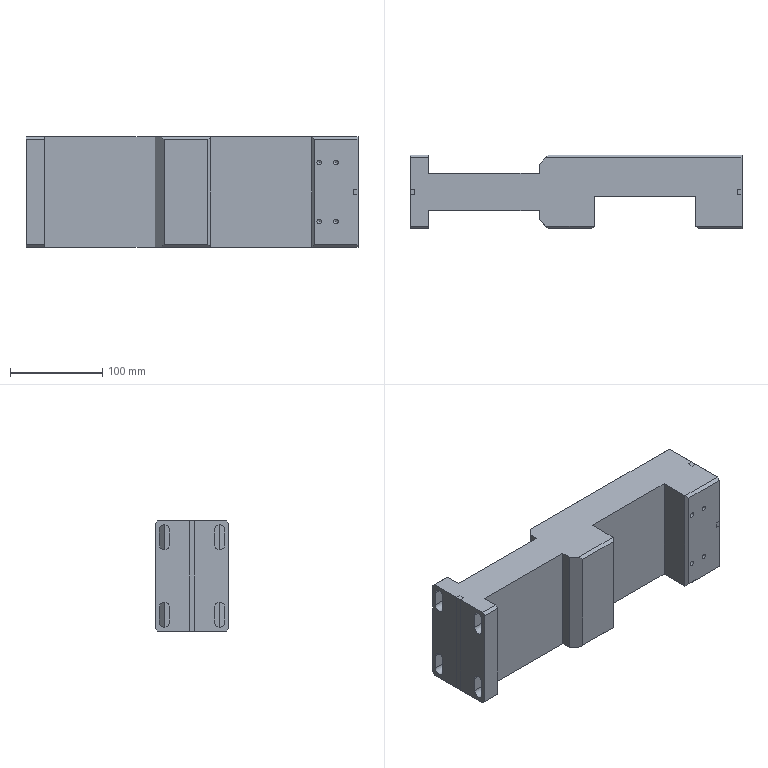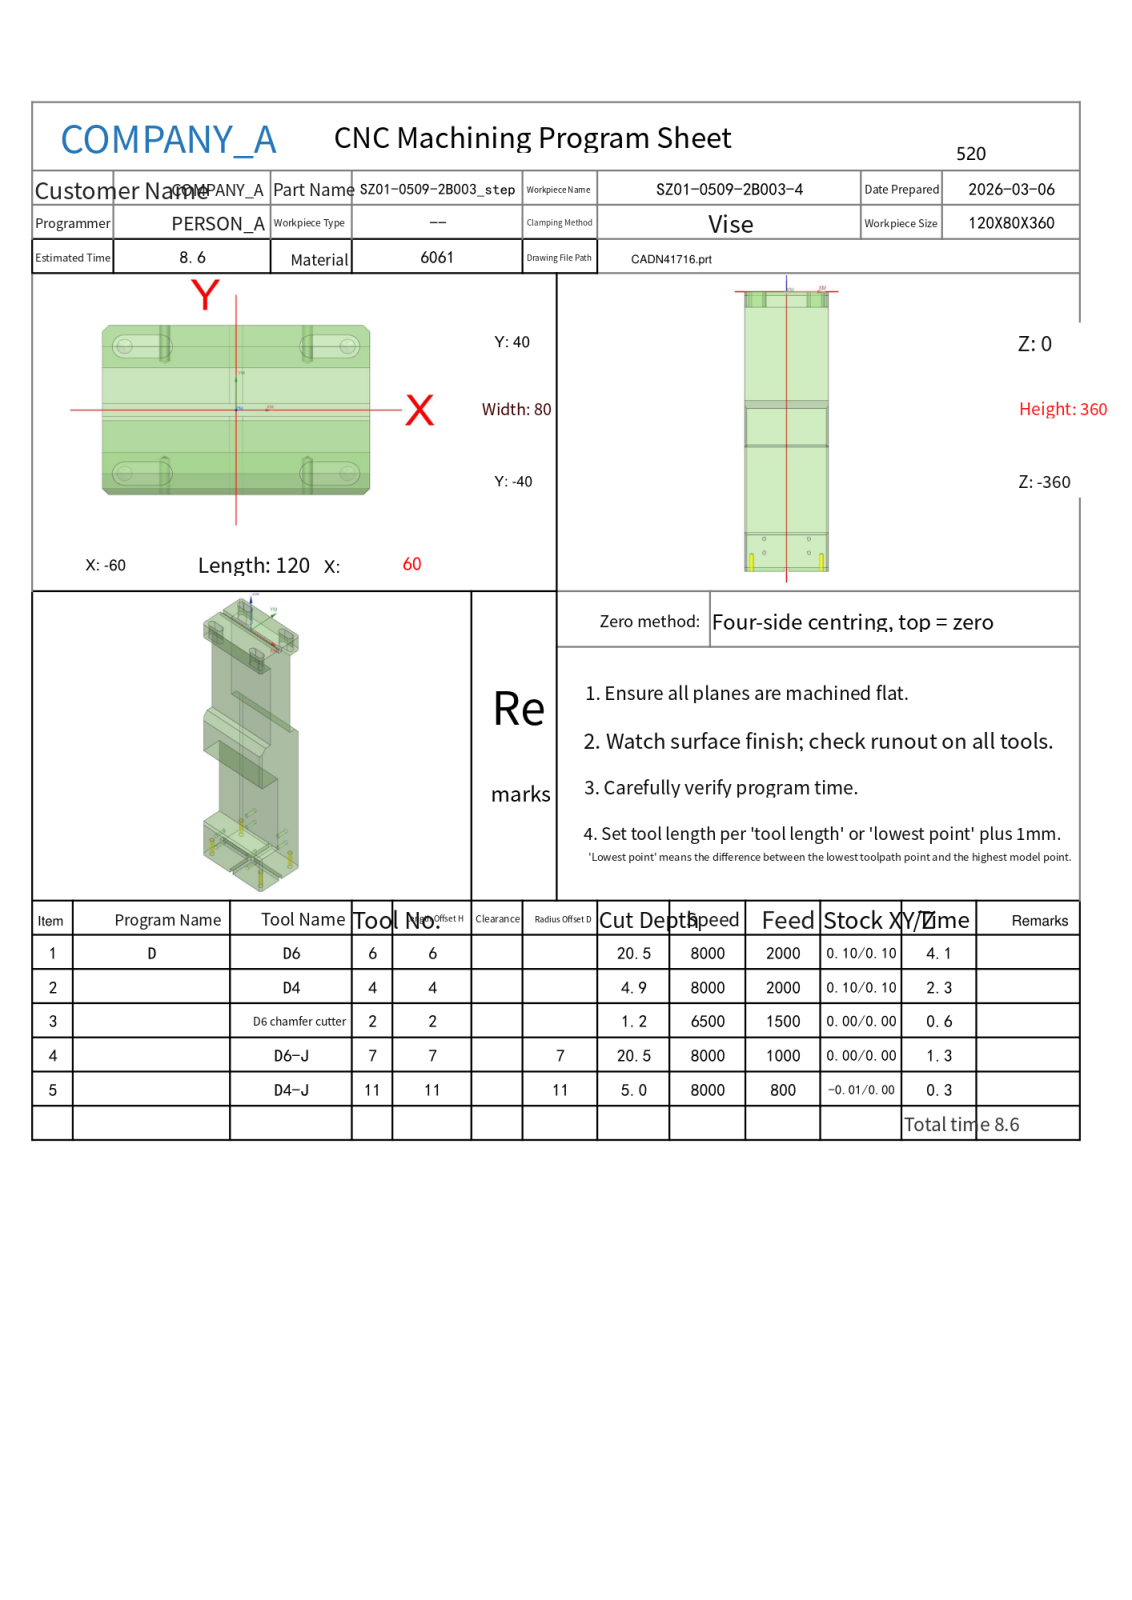NC program | NX | posted by the shop | part box 360 x 80 x 120 mm
Whole program, first 1404 of 1841 lines:
%
O0001
(Machine time: 9.60 MIN)
(===Total Tool:5===)
(T6=D6      D=6.   R=0.   D-  H06 Z=-20.5 )
(T4=D4      D=4.   R=0.   D-  H04 Z=-4.9  )
(T2=D6 chamfer cutter   D=6.   R=0.   D-  H02 Z=-1.2  )
(T7=D6-J    D=6.   R=0.   D7  H07 Z=-20.5 )
(T11=D4-J   D=4.   R=0.   D11 H11 Z=-5.   )
G80 G90 G17 G49 G40
G91 G28 Z0
M01
N1 T06 M06
(D6  D=6. R=0. H=06 ce=0.10 di=0.10)
G00 G90 G54 X-38.502 Y-27.6 M03 S8000
G43 H06 Z50.
M08
Z1.
G01 X-50.381 Z.377 F2000.
X-51.324 Y-27.962 Z.325
X-52.038 Y-28.676 Z.272
X-52.4 Y-29.619 Z.219
Y-30.381 Z.179
X-52.038 Y-31.324 Z.126
X-51.324 Y-32.038 Z.073
X-50.381 Y-32.4 Z.02
X-50. Z0.0
X-34. Z-.166
G03 X-31.6 Y-30. Z-.205 I0.0 J2.4
X-34. Y-27.6 Z-.244 I-2.4 J0.0
G01 X-50. Z-.41
G03 X-52.4 Y-30. Z-.449 I0.0 J-2.4
X-50. Y-32.4 Z-.488 I2.4 J0.0
G01 X-34. Z-.654
G03 X-31.6 Y-30. Z-.693 I0.0 J2.4
X-34. Y-27.6 Z-.732 I-2.4 J0.0
G01 X-50. Z-.898
G03 X-52.4 Y-30. Z-.937 I0.0 J-2.4
X-50. Y-32.4 Z-.976 I2.4 J0.0
G01 X-34. Z-1.142
G03 X-31.6 Y-30. Z-1.181 I0.0 J2.4
X-34. Y-27.6 Z-1.22 I-2.4 J0.0
G01 X-50. Z-1.386
G03 X-52.4 Y-30. Z-1.425 I0.0 J-2.4
X-50. Y-32.4 Z-1.464 I2.4 J0.0
G01 X-34. Z-1.63
G03 X-31.6 Y-30. Z-1.669 I0.0 J2.4
X-34. Y-27.6 Z-1.708 I-2.4 J0.0
G01 X-50. Z-1.874
G03 X-52.4 Y-30. Z-1.913 I0.0 J-2.4
X-50. Y-32.4 Z-1.952 I2.4 J0.0
G01 X-34. Z-2.118
G03 X-31.6 Y-30. Z-2.157 I0.0 J2.4
X-34. Y-27.6 Z-2.196 I-2.4 J0.0
G01 X-50. Z-2.362
G03 X-52.4 Y-30. Z-2.401 I0.0 J-2.4
X-50. Y-32.4 Z-2.44 I2.4 J0.0
G01 X-34. Z-2.606
G03 X-31.6 Y-30. Z-2.645 I0.0 J2.4
X-34. Y-27.6 Z-2.685 I-2.4 J0.0
G01 X-50. Z-2.85
G03 X-52.4 Y-30. Z-2.889 I0.0 J-2.4
X-50. Y-32.4 Z-2.929 I2.4 J0.0
G01 X-34. Z-3.094
G03 X-31.6 Y-30. Z-3.134 I0.0 J2.4
X-34. Y-27.6 Z-3.173 I-2.4 J0.0
G01 X-50. Z-3.338
G03 X-52.4 Y-30. Z-3.378 I0.0 J-2.4
X-50. Y-32.4 Z-3.417 I2.4 J0.0
G01 X-34. Z-3.583
G03 X-31.6 Y-30. Z-3.622 I0.0 J2.4
X-34. Y-27.6 Z-3.661 I-2.4 J0.0
G01 X-50. Z-3.827
G03 X-52.4 Y-30. Z-3.866 I0.0 J-2.4
X-50. Y-32.4 Z-3.905 I2.4 J0.0
G01 X-34. Z-4.071
G03 X-31.6 Y-30. Z-4.11 I0.0 J2.4
X-34. Y-27.6 Z-4.149 I-2.4 J0.0
G01 X-50. Z-4.315
G03 X-52.4 Y-30. Z-4.354 I0.0 J-2.4
X-50. Y-32.4 Z-4.393 I2.4 J0.0
G01 X-34. Z-4.559
G03 X-31.6 Y-30. Z-4.598 I0.0 J2.4
X-34. Y-27.6 Z-4.637 I-2.4 J0.0
G01 X-50. Z-4.803
G03 X-52.4 Y-30. Z-4.842 I0.0 J-2.4
X-50. Y-32.4 Z-4.881 I2.4 J0.0
G01 X-34. Z-5.047
G03 X-31.6 Y-30. Z-5.086 I0.0 J2.4
X-34. Y-27.6 Z-5.125 I-2.4 J0.0
G01 X-50. Z-5.291
G03 X-52.4 Y-30. Z-5.33 I0.0 J-2.4
X-50. Y-32.4 Z-5.369 I2.4 J0.0
G01 X-34. Z-5.535
G03 X-31.6 Y-30. Z-5.574 I0.0 J2.4
X-34. Y-27.6 Z-5.613 I-2.4 J0.0
G01 X-50. Z-5.779
G03 X-52.4 Y-30. Z-5.818 I0.0 J-2.4
X-50. Y-32.4 Z-5.857 I2.4 J0.0
G01 X-34. Z-6.023
G03 X-31.6 Y-30. Z-6.062 I0.0 J2.4
X-34. Y-27.6 Z-6.101 I-2.4 J0.0
G01 X-50. Z-6.267
G03 X-52.4 Y-30. Z-6.306 I0.0 J-2.4
X-50. Y-32.4 Z-6.345 I2.4 J0.0
G01 X-34. Z-6.511
G03 X-31.6 Y-30. Z-6.55 I0.0 J2.4
X-34. Y-27.6 Z-6.589 I-2.4 J0.0
G01 X-50. Z-6.755
G03 X-52.4 Y-30. Z-6.794 I0.0 J-2.4
X-50. Y-32.4 Z-6.833 I2.4 J0.0
G01 X-34. Z-6.999
G03 X-31.6 Y-30. Z-7.038 I0.0 J2.4
X-34. Y-27.6 Z-7.077 I-2.4 J0.0
G01 X-50. Z-7.243
G03 X-52.4 Y-30. Z-7.282 I0.0 J-2.4
X-50. Y-32.4 Z-7.321 I2.4 J0.0
G01 X-34. Z-7.487
G03 X-31.6 Y-30. Z-7.526 I0.0 J2.4
X-34. Y-27.6 Z-7.565 I-2.4 J0.0
G01 X-50. Z-7.731
G03 X-52.4 Y-30. Z-7.77 I0.0 J-2.4
X-50. Y-32.4 Z-7.81 I2.4 J0.0
G01 X-34. Z-7.975
G03 X-31.6 Y-30. Z-8.014 I0.0 J2.4
X-34. Y-27.6 Z-8.054 I-2.4 J0.0
G01 X-50. Z-8.219
G03 X-52.4 Y-30. Z-8.259 I0.0 J-2.4
X-50. Y-32.4 Z-8.298 I2.4 J0.0
G01 X-34. Z-8.463
G03 X-31.6 Y-30. Z-8.503 I0.0 J2.4
X-34. Y-27.6 Z-8.542 I-2.4 J0.0
G01 X-50. Z-8.708
G03 X-52.4 Y-30. Z-8.747 I0.0 J-2.4
X-50. Y-32.4 Z-8.786 I2.4 J0.0
G01 X-34. Z-8.952
G03 X-31.6 Y-30. Z-8.991 I0.0 J2.4
X-34. Y-27.6 Z-9.03 I-2.4 J0.0
G01 X-50. Z-9.196
G03 X-52.4 Y-30. Z-9.235 I0.0 J-2.4
X-50. Y-32.4 Z-9.274 I2.4 J0.0
G01 X-34. Z-9.44
G03 X-31.6 Y-30. Z-9.479 I0.0 J2.4
X-34. Y-27.6 Z-9.518 I-2.4 J0.0
G01 X-50. Z-9.684
G03 X-52.4 Y-30. Z-9.723 I0.0 J-2.4
X-50. Y-32.4 Z-9.762 I2.4 J0.0
G01 X-34. Z-9.928
G03 X-31.6 Y-30. Z-9.967 I0.0 J2.4
X-34. Y-27.6 Z-10.006 I-2.4 J0.0
G01 X-50. Z-10.172
G03 X-52.4 Y-30. Z-10.211 I0.0 J-2.4
X-50. Y-32.4 Z-10.25 I2.4 J0.0
G01 X-34. Z-10.416
G03 X-31.6 Y-30. Z-10.455 I0.0 J2.4
X-34. Y-27.6 Z-10.494 I-2.4 J0.0
G01 X-50. Z-10.66
G03 X-52.4 Y-30. Z-10.699 I0.0 J-2.4
X-50. Y-32.4 Z-10.738 I2.4 J0.0
G01 X-34. Z-10.904
G03 X-31.6 Y-30. Z-10.943 I0.0 J2.4
X-34. Y-27.6 Z-10.982 I-2.4 J0.0
G01 X-50. Z-11.148
G03 X-52.4 Y-30. Z-11.187 I0.0 J-2.4
X-50. Y-32.4 Z-11.226 I2.4 J0.0
G01 X-34. Z-11.392
G03 X-31.6 Y-30. Z-11.431 I0.0 J2.4
X-34. Y-27.6 Z-11.47 I-2.4 J0.0
G01 X-50. Z-11.636
G03 X-52.4 Y-30. Z-11.675 I0.0 J-2.4
X-50. Y-32.4 Z-11.714 I2.4 J0.0
G01 X-34. Z-11.88
G03 X-31.6 Y-30. Z-11.919 I0.0 J2.4
X-34. Y-27.6 Z-11.958 I-2.4 J0.0
G01 X-50. Z-12.124
G03 X-52.4 Y-30. Z-12.163 I0.0 J-2.4
X-50. Y-32.4 Z-12.202 I2.4 J0.0
G01 X-34. Z-12.368
G03 X-31.6 Y-30. Z-12.407 I0.0 J2.4
X-34. Y-27.6 Z-12.446 I-2.4 J0.0
G01 X-50. Z-12.612
G03 X-52.4 Y-30. Z-12.651 I0.0 J-2.4
X-50. Y-32.4 Z-12.69 I2.4 J0.0
G01 X-34. Z-12.856
G03 X-31.6 Y-30. Z-12.895 I0.0 J2.4
X-34. Y-27.6 Z-12.935 I-2.4 J0.0
G01 X-50. Z-13.1
G03 X-52.4 Y-30. Z-13.139 I0.0 J-2.4
X-50. Y-32.4 Z-13.179 I2.4 J0.0
G01 X-34. Z-13.344
G03 X-31.6 Y-30. Z-13.384 I0.0 J2.4
X-34. Y-27.6 Z-13.423 I-2.4 J0.0
G01 X-50. Z-13.588
G03 X-52.4 Y-30. Z-13.628 I0.0 J-2.4
X-50. Y-32.4 Z-13.667 I2.4 J0.0
G01 X-34. Z-13.833
G03 X-31.6 Y-30. Z-13.872 I0.0 J2.4
X-34. Y-27.6 Z-13.911 I-2.4 J0.0
G01 X-50. Z-14.077
G03 X-52.4 Y-30. Z-14.116 I0.0 J-2.4
X-50. Y-32.4 Z-14.155 I2.4 J0.0
G01 X-34. Z-14.321
G03 X-31.6 Y-30. Z-14.36 I0.0 J2.4
X-34. Y-27.6 Z-14.399 I-2.4 J0.0
G01 X-50. Z-14.565
G03 X-52.4 Y-30. Z-14.604 I0.0 J-2.4
X-50. Y-32.4 Z-14.643 I2.4 J0.0
G01 X-34. Z-14.809
G03 X-31.6 Y-30. Z-14.848 I0.0 J2.4
X-34. Y-27.6 Z-14.887 I-2.4 J0.0
G01 X-50. Z-15.053
G03 X-52.4 Y-30. Z-15.092 I0.0 J-2.4
X-50. Y-32.4 Z-15.131 I2.4 J0.0
G01 X-34. Z-15.297
G03 X-31.6 Y-30. Z-15.336 I0.0 J2.4
X-34. Y-27.6 Z-15.375 I-2.4 J0.0
G01 X-50. Z-15.541
G03 X-52.4 Y-30. Z-15.58 I0.0 J-2.4
X-50. Y-32.4 Z-15.619 I2.4 J0.0
G01 X-34. Z-15.785
G03 X-31.6 Y-30. Z-15.824 I0.0 J2.4
X-34. Y-27.6 Z-15.863 I-2.4 J0.0
G01 X-50. Z-16.029
G03 X-52.4 Y-30. Z-16.068 I0.0 J-2.4
X-50. Y-32.4 Z-16.107 I2.4 J0.0
G01 X-34. Z-16.273
G03 X-31.6 Y-30. Z-16.312 I0.0 J2.4
X-34. Y-27.6 Z-16.351 I-2.4 J0.0
G01 X-50. Z-16.517
G03 X-52.4 Y-30. Z-16.556 I0.0 J-2.4
X-50. Y-32.4 Z-16.595 I2.4 J0.0
G01 X-34. Z-16.761
G03 X-31.6 Y-30. Z-16.8 I0.0 J2.4
X-34. Y-27.6 Z-16.839 I-2.4 J0.0
G01 X-50. Z-17.005
G03 X-52.4 Y-30. Z-17.044 I0.0 J-2.4
X-50. Y-32.4 Z-17.083 I2.4 J0.0
G01 X-34. Z-17.249
G03 X-31.6 Y-30. Z-17.288 I0.0 J2.4
X-34. Y-27.6 Z-17.327 I-2.4 J0.0
G01 X-50. Z-17.493
G03 X-52.4 Y-30. Z-17.532 I0.0 J-2.4
X-50. Y-32.4 Z-17.571 I2.4 J0.0
G01 X-34. Z-17.737
G03 X-31.6 Y-30. Z-17.776 I0.0 J2.4
X-34. Y-27.6 Z-17.815 I-2.4 J0.0
G01 X-50. Z-17.981
G03 X-52.4 Y-30. Z-18.02 I0.0 J-2.4
X-50. Y-32.4 Z-18.06 I2.4 J0.0
G01 X-34. Z-18.225
G03 X-31.6 Y-30. Z-18.264 I0.0 J2.4
X-34. Y-27.6 Z-18.304 I-2.4 J0.0
G01 X-50. Z-18.469
G03 X-52.4 Y-30. Z-18.509 I0.0 J-2.4
X-50. Y-32.4 Z-18.548 I2.4 J0.0
G01 X-34. Z-18.713
G03 X-31.6 Y-30. Z-18.753 I0.0 J2.4
X-34. Y-27.6 Z-18.792 I-2.4 J0.0
G01 X-50. Z-18.958
G03 X-52.4 Y-30. Z-18.997 I0.0 J-2.4
X-50. Y-32.4 Z-19.036 I2.4 J0.0
G01 X-34. Z-19.202
G03 X-31.6 Y-30. Z-19.241 I0.0 J2.4
X-34. Y-27.6 Z-19.28 I-2.4 J0.0
G01 X-50. Z-19.446
G03 X-52.4 Y-30. Z-19.485 I0.0 J-2.4
X-50. Y-32.4 Z-19.524 I2.4 J0.0
G01 X-34. Z-19.69
G03 X-31.6 Y-30. Z-19.729 I0.0 J2.4
X-34. Y-27.6 Z-19.768 I-2.4 J0.0
G01 X-50. Z-19.934
G03 X-52.4 Y-30. Z-19.973 I0.0 J-2.4
X-50. Y-32.4 Z-20.012 I2.4 J0.0
G01 X-34. Z-20.178
G03 X-31.6 Y-30. Z-20.217 I0.0 J2.4
X-34. Y-27.6 Z-20.256 I-2.4 J0.0
G01 X-50. Z-20.422
G03 X-52.4 Y-30. Z-20.461 I0.0 J-2.4
X-50. Y-32.4 Z-20.5 I2.4 J0.0
G01 X-34.
G03 X-31.6 Y-30. I0.0 J2.4
X-34. Y-27.6 I-2.4 J0.0
G01 X-50.
G03 X-52.4 Y-30. I0.0 J-2.4
X-50. Y-32.4 I2.4 J0.0
G01 X-49.6
Z-19.5
G00 Z50.
X-45.498 Y27.6
Z1.
G01 X-33.619 Z.377
X-32.676 Y27.962 Z.325
X-31.962 Y28.676 Z.272
X-31.6 Y29.619 Z.219
Y30.381 Z.179
X-31.962 Y31.324 Z.126
X-32.676 Y32.038 Z.073
X-33.619 Y32.4 Z.02
X-34. Z0.0
X-50. Z-.166
G03 X-52.4 Y30. Z-.205 I0.0 J-2.4
X-50. Y27.6 Z-.244 I2.4 J0.0
G01 X-34. Z-.41
G03 X-31.6 Y30. Z-.449 I0.0 J2.4
X-34. Y32.4 Z-.488 I-2.4 J0.0
G01 X-50. Z-.654
G03 X-52.4 Y30. Z-.693 I0.0 J-2.4
X-50. Y27.6 Z-.732 I2.4 J0.0
G01 X-34. Z-.898
G03 X-31.6 Y30. Z-.937 I0.0 J2.4
X-34. Y32.4 Z-.976 I-2.4 J0.0
G01 X-50. Z-1.142
G03 X-52.4 Y30. Z-1.181 I0.0 J-2.4
X-50. Y27.6 Z-1.22 I2.4 J0.0
G01 X-34. Z-1.386
G03 X-31.6 Y30. Z-1.425 I0.0 J2.4
X-34. Y32.4 Z-1.464 I-2.4 J0.0
G01 X-50. Z-1.63
G03 X-52.4 Y30. Z-1.669 I0.0 J-2.4
X-50. Y27.6 Z-1.708 I2.4 J0.0
G01 X-34. Z-1.874
G03 X-31.6 Y30. Z-1.913 I0.0 J2.4
X-34. Y32.4 Z-1.952 I-2.4 J0.0
G01 X-50. Z-2.118
G03 X-52.4 Y30. Z-2.157 I0.0 J-2.4
X-50. Y27.6 Z-2.196 I2.4 J0.0
G01 X-34. Z-2.362
G03 X-31.6 Y30. Z-2.401 I0.0 J2.4
X-34. Y32.4 Z-2.44 I-2.4 J0.0
G01 X-50. Z-2.606
G03 X-52.4 Y30. Z-2.645 I0.0 J-2.4
X-50. Y27.6 Z-2.685 I2.4 J0.0
G01 X-34. Z-2.85
G03 X-31.6 Y30. Z-2.889 I0.0 J2.4
X-34. Y32.4 Z-2.929 I-2.4 J0.0
G01 X-50. Z-3.094
G03 X-52.4 Y30. Z-3.134 I0.0 J-2.4
X-50. Y27.6 Z-3.173 I2.4 J0.0
G01 X-34. Z-3.338
G03 X-31.6 Y30. Z-3.378 I0.0 J2.4
X-34. Y32.4 Z-3.417 I-2.4 J0.0
G01 X-50. Z-3.583
G03 X-52.4 Y30. Z-3.622 I0.0 J-2.4
X-50. Y27.6 Z-3.661 I2.4 J0.0
G01 X-34. Z-3.827
G03 X-31.6 Y30. Z-3.866 I0.0 J2.4
X-34. Y32.4 Z-3.905 I-2.4 J0.0
G01 X-50. Z-4.071
G03 X-52.4 Y30. Z-4.11 I0.0 J-2.4
X-50. Y27.6 Z-4.149 I2.4 J0.0
G01 X-34. Z-4.315
G03 X-31.6 Y30. Z-4.354 I0.0 J2.4
X-34. Y32.4 Z-4.393 I-2.4 J0.0
G01 X-50. Z-4.559
G03 X-52.4 Y30. Z-4.598 I0.0 J-2.4
X-50. Y27.6 Z-4.637 I2.4 J0.0
G01 X-34. Z-4.803
G03 X-31.6 Y30. Z-4.842 I0.0 J2.4
X-34. Y32.4 Z-4.881 I-2.4 J0.0
G01 X-50. Z-5.047
G03 X-52.4 Y30. Z-5.086 I0.0 J-2.4
X-50. Y27.6 Z-5.125 I2.4 J0.0
G01 X-34. Z-5.291
G03 X-31.6 Y30. Z-5.33 I0.0 J2.4
X-34. Y32.4 Z-5.369 I-2.4 J0.0
G01 X-50. Z-5.535
G03 X-52.4 Y30. Z-5.574 I0.0 J-2.4
X-50. Y27.6 Z-5.613 I2.4 J0.0
G01 X-34. Z-5.779
G03 X-31.6 Y30. Z-5.818 I0.0 J2.4
X-34. Y32.4 Z-5.857 I-2.4 J0.0
G01 X-50. Z-6.023
G03 X-52.4 Y30. Z-6.062 I0.0 J-2.4
X-50. Y27.6 Z-6.101 I2.4 J0.0
G01 X-34. Z-6.267
G03 X-31.6 Y30. Z-6.306 I0.0 J2.4
X-34. Y32.4 Z-6.345 I-2.4 J0.0
G01 X-50. Z-6.511
G03 X-52.4 Y30. Z-6.55 I0.0 J-2.4
X-50. Y27.6 Z-6.589 I2.4 J0.0
G01 X-34. Z-6.755
G03 X-31.6 Y30. Z-6.794 I0.0 J2.4
X-34. Y32.4 Z-6.833 I-2.4 J0.0
G01 X-50. Z-6.999
G03 X-52.4 Y30. Z-7.038 I0.0 J-2.4
X-50. Y27.6 Z-7.077 I2.4 J0.0
G01 X-34. Z-7.243
G03 X-31.6 Y30. Z-7.282 I0.0 J2.4
X-34. Y32.4 Z-7.321 I-2.4 J0.0
G01 X-50. Z-7.487
G03 X-52.4 Y30. Z-7.526 I0.0 J-2.4
X-50. Y27.6 Z-7.565 I2.4 J0.0
G01 X-34. Z-7.731
G03 X-31.6 Y30. Z-7.77 I0.0 J2.4
X-34. Y32.4 Z-7.81 I-2.4 J0.0
G01 X-50. Z-7.975
G03 X-52.4 Y30. Z-8.014 I0.0 J-2.4
X-50. Y27.6 Z-8.054 I2.4 J0.0
G01 X-34. Z-8.219
G03 X-31.6 Y30. Z-8.259 I0.0 J2.4
X-34. Y32.4 Z-8.298 I-2.4 J0.0
G01 X-50. Z-8.463
G03 X-52.4 Y30. Z-8.503 I0.0 J-2.4
X-50. Y27.6 Z-8.542 I2.4 J0.0
G01 X-34. Z-8.708
G03 X-31.6 Y30. Z-8.747 I0.0 J2.4
X-34. Y32.4 Z-8.786 I-2.4 J0.0
G01 X-50. Z-8.952
G03 X-52.4 Y30. Z-8.991 I0.0 J-2.4
X-50. Y27.6 Z-9.03 I2.4 J0.0
G01 X-34. Z-9.196
G03 X-31.6 Y30. Z-9.235 I0.0 J2.4
X-34. Y32.4 Z-9.274 I-2.4 J0.0
G01 X-50. Z-9.44
G03 X-52.4 Y30. Z-9.479 I0.0 J-2.4
X-50. Y27.6 Z-9.518 I2.4 J0.0
G01 X-34. Z-9.684
G03 X-31.6 Y30. Z-9.723 I0.0 J2.4
X-34. Y32.4 Z-9.762 I-2.4 J0.0
G01 X-50. Z-9.928
G03 X-52.4 Y30. Z-9.967 I0.0 J-2.4
X-50. Y27.6 Z-10.006 I2.4 J0.0
G01 X-34. Z-10.172
G03 X-31.6 Y30. Z-10.211 I0.0 J2.4
X-34. Y32.4 Z-10.25 I-2.4 J0.0
G01 X-50. Z-10.416
G03 X-52.4 Y30. Z-10.455 I0.0 J-2.4
X-50. Y27.6 Z-10.494 I2.4 J0.0
G01 X-34. Z-10.66
G03 X-31.6 Y30. Z-10.699 I0.0 J2.4
X-34. Y32.4 Z-10.738 I-2.4 J0.0
G01 X-50. Z-10.904
G03 X-52.4 Y30. Z-10.943 I0.0 J-2.4
X-50. Y27.6 Z-10.982 I2.4 J0.0
G01 X-34. Z-11.148
G03 X-31.6 Y30. Z-11.187 I0.0 J2.4
X-34. Y32.4 Z-11.226 I-2.4 J0.0
G01 X-50. Z-11.392
G03 X-52.4 Y30. Z-11.431 I0.0 J-2.4
X-50. Y27.6 Z-11.47 I2.4 J0.0
G01 X-34. Z-11.636
G03 X-31.6 Y30. Z-11.675 I0.0 J2.4
X-34. Y32.4 Z-11.714 I-2.4 J0.0
G01 X-50. Z-11.88
G03 X-52.4 Y30. Z-11.919 I0.0 J-2.4
X-50. Y27.6 Z-11.958 I2.4 J0.0
G01 X-34. Z-12.124
G03 X-31.6 Y30. Z-12.163 I0.0 J2.4
X-34. Y32.4 Z-12.202 I-2.4 J0.0
G01 X-50. Z-12.368
G03 X-52.4 Y30. Z-12.407 I0.0 J-2.4
X-50. Y27.6 Z-12.446 I2.4 J0.0
G01 X-34. Z-12.612
G03 X-31.6 Y30. Z-12.651 I0.0 J2.4
X-34. Y32.4 Z-12.69 I-2.4 J0.0
G01 X-50. Z-12.856
G03 X-52.4 Y30. Z-12.895 I0.0 J-2.4
X-50. Y27.6 Z-12.935 I2.4 J0.0
G01 X-34. Z-13.1
G03 X-31.6 Y30. Z-13.139 I0.0 J2.4
X-34. Y32.4 Z-13.179 I-2.4 J0.0
G01 X-50. Z-13.344
G03 X-52.4 Y30. Z-13.384 I0.0 J-2.4
X-50. Y27.6 Z-13.423 I2.4 J0.0
G01 X-34. Z-13.588
G03 X-31.6 Y30. Z-13.628 I0.0 J2.4
X-34. Y32.4 Z-13.667 I-2.4 J0.0
G01 X-50. Z-13.833
G03 X-52.4 Y30. Z-13.872 I0.0 J-2.4
X-50. Y27.6 Z-13.911 I2.4 J0.0
G01 X-34. Z-14.077
G03 X-31.6 Y30. Z-14.116 I0.0 J2.4
X-34. Y32.4 Z-14.155 I-2.4 J0.0
G01 X-50. Z-14.321
G03 X-52.4 Y30. Z-14.36 I0.0 J-2.4
X-50. Y27.6 Z-14.399 I2.4 J0.0
G01 X-34. Z-14.565
G03 X-31.6 Y30. Z-14.604 I0.0 J2.4
X-34. Y32.4 Z-14.643 I-2.4 J0.0
G01 X-50. Z-14.809
G03 X-52.4 Y30. Z-14.848 I0.0 J-2.4
X-50. Y27.6 Z-14.887 I2.4 J0.0
G01 X-34. Z-15.053
G03 X-31.6 Y30. Z-15.092 I0.0 J2.4
X-34. Y32.4 Z-15.131 I-2.4 J0.0
G01 X-50. Z-15.297
G03 X-52.4 Y30. Z-15.336 I0.0 J-2.4
X-50. Y27.6 Z-15.375 I2.4 J0.0
G01 X-34. Z-15.541
G03 X-31.6 Y30. Z-15.58 I0.0 J2.4
X-34. Y32.4 Z-15.619 I-2.4 J0.0
G01 X-50. Z-15.785
G03 X-52.4 Y30. Z-15.824 I0.0 J-2.4
X-50. Y27.6 Z-15.863 I2.4 J0.0
G01 X-34. Z-16.029
G03 X-31.6 Y30. Z-16.068 I0.0 J2.4
X-34. Y32.4 Z-16.107 I-2.4 J0.0
G01 X-50. Z-16.273
G03 X-52.4 Y30. Z-16.312 I0.0 J-2.4
X-50. Y27.6 Z-16.351 I2.4 J0.0
G01 X-34. Z-16.517
G03 X-31.6 Y30. Z-16.556 I0.0 J2.4
X-34. Y32.4 Z-16.595 I-2.4 J0.0
G01 X-50. Z-16.761
G03 X-52.4 Y30. Z-16.8 I0.0 J-2.4
X-50. Y27.6 Z-16.839 I2.4 J0.0
G01 X-34. Z-17.005
G03 X-31.6 Y30. Z-17.044 I0.0 J2.4
X-34. Y32.4 Z-17.083 I-2.4 J0.0
G01 X-50. Z-17.249
G03 X-52.4 Y30. Z-17.288 I0.0 J-2.4
X-50. Y27.6 Z-17.327 I2.4 J0.0
G01 X-34. Z-17.493
G03 X-31.6 Y30. Z-17.532 I0.0 J2.4
X-34. Y32.4 Z-17.571 I-2.4 J0.0
G01 X-50. Z-17.737
G03 X-52.4 Y30. Z-17.776 I0.0 J-2.4
X-50. Y27.6 Z-17.815 I2.4 J0.0
G01 X-34. Z-17.981
G03 X-31.6 Y30. Z-18.02 I0.0 J2.4
X-34. Y32.4 Z-18.06 I-2.4 J0.0
G01 X-50. Z-18.225
G03 X-52.4 Y30. Z-18.264 I0.0 J-2.4
X-50. Y27.6 Z-18.304 I2.4 J0.0
G01 X-34. Z-18.469
G03 X-31.6 Y30. Z-18.509 I0.0 J2.4
X-34. Y32.4 Z-18.548 I-2.4 J0.0
G01 X-50. Z-18.713
G03 X-52.4 Y30. Z-18.753 I0.0 J-2.4
X-50. Y27.6 Z-18.792 I2.4 J0.0
G01 X-34. Z-18.958
G03 X-31.6 Y30. Z-18.997 I0.0 J2.4
X-34. Y32.4 Z-19.036 I-2.4 J0.0
G01 X-50. Z-19.202
G03 X-52.4 Y30. Z-19.241 I0.0 J-2.4
X-50. Y27.6 Z-19.28 I2.4 J0.0
G01 X-34. Z-19.446
G03 X-31.6 Y30. Z-19.485 I0.0 J2.4
X-34. Y32.4 Z-19.524 I-2.4 J0.0
G01 X-50. Z-19.69
G03 X-52.4 Y30. Z-19.729 I0.0 J-2.4
X-50. Y27.6 Z-19.768 I2.4 J0.0
G01 X-34. Z-19.934
G03 X-31.6 Y30. Z-19.973 I0.0 J2.4
X-34. Y32.4 Z-20.012 I-2.4 J0.0
G01 X-50. Z-20.178
G03 X-52.4 Y30. Z-20.217 I0.0 J-2.4
X-50. Y27.6 Z-20.256 I2.4 J0.0
G01 X-34. Z-20.422
G03 X-31.6 Y30. Z-20.461 I0.0 J2.4
X-34. Y32.4 Z-20.5 I-2.4 J0.0
G01 X-50.
G03 X-52.4 Y30. I0.0 J-2.4
X-50. Y27.6 I2.4 J0.0
G01 X-34.
G03 X-31.6 Y30. I0.0 J2.4
X-34. Y32.4 I-2.4 J0.0
G01 X-34.4
Z-19.5
G00 Z50.
X38.502 Y27.6
Z1.
G01 X50.381 Z.377
X51.324 Y27.962 Z.325
X52.038 Y28.676 Z.272
X52.4 Y29.619 Z.219
Y30.381 Z.179
X52.038 Y31.324 Z.126
X51.324 Y32.038 Z.073
X50.381 Y32.4 Z.02
X50. Z0.0
X34. Z-.17
G03 X31.6 Y30. Z-.21 I0.0 J-2.4
X34. Y27.6 Z-.25 I2.4 J0.0
G01 X50. Z-.42
G03 X52.4 Y30. Z-.46 I0.0 J2.4
X50. Y32.4 Z-.5 I-2.4 J0.0
G01 X34. Z-.67
G03 X31.6 Y30. Z-.71 I0.0 J-2.4
X34. Y27.6 Z-.75 I2.4 J0.0
G01 X50. Z-.92
G03 X52.4 Y30. Z-.96 I0.0 J2.4
X50. Y32.4 Z-1. I-2.4 J0.0
G01 X34. Z-1.17
G03 X31.6 Y30. Z-1.21 I0.0 J-2.4
X34. Y27.6 Z-1.25 I2.4 J0.0
G01 X50. Z-1.42
G03 X52.4 Y30. Z-1.46 I0.0 J2.4
X50. Y32.4 Z-1.5 I-2.4 J0.0
G01 X34. Z-1.67
G03 X31.6 Y30. Z-1.71 I0.0 J-2.4
X34. Y27.6 Z-1.75 I2.4 J0.0
G01 X50. Z-1.92
G03 X52.4 Y30. Z-1.96 I0.0 J2.4
X50. Y32.4 Z-2. I-2.4 J0.0
G01 X34. Z-2.17
G03 X31.6 Y30. Z-2.21 I0.0 J-2.4
X34. Y27.6 Z-2.25 I2.4 J0.0
G01 X50. Z-2.42
G03 X52.4 Y30. Z-2.46 I0.0 J2.4
X50. Y32.4 Z-2.5 I-2.4 J0.0
G01 X34. Z-2.67
G03 X31.6 Y30. Z-2.71 I0.0 J-2.4
X34. Y27.6 Z-2.75 I2.4 J0.0
G01 X50. Z-2.92
G03 X52.4 Y30. Z-2.96 I0.0 J2.4
X50. Y32.4 Z-3. I-2.4 J0.0
G01 X34. Z-3.17
G03 X31.6 Y30. Z-3.21 I0.0 J-2.4
X34. Y27.6 Z-3.25 I2.4 J0.0
G01 X50. Z-3.42
G03 X52.4 Y30. Z-3.46 I0.0 J2.4
X50. Y32.4 Z-3.5 I-2.4 J0.0
G01 X34. Z-3.67
G03 X31.6 Y30. Z-3.71 I0.0 J-2.4
X34. Y27.6 Z-3.75 I2.4 J0.0
G01 X50. Z-3.92
G03 X52.4 Y30. Z-3.96 I0.0 J2.4
X50. Y32.4 Z-4. I-2.4 J0.0
G01 X34. Z-4.17
G03 X31.6 Y30. Z-4.21 I0.0 J-2.4
X34. Y27.6 Z-4.25 I2.4 J0.0
G01 X50. Z-4.42
G03 X52.4 Y30. Z-4.46 I0.0 J2.4
X50. Y32.4 Z-4.5 I-2.4 J0.0
G01 X34. Z-4.67
G03 X31.6 Y30. Z-4.71 I0.0 J-2.4
X34. Y27.6 Z-4.75 I2.4 J0.0
G01 X50. Z-4.92
G03 X52.4 Y30. Z-4.96 I0.0 J2.4
X50. Y32.4 Z-5. I-2.4 J0.0
G01 X34. Z-5.17
G03 X31.6 Y30. Z-5.21 I0.0 J-2.4
X34. Y27.6 Z-5.25 I2.4 J0.0
G01 X50. Z-5.42
G03 X52.4 Y30. Z-5.46 I0.0 J2.4
X50. Y32.4 Z-5.5 I-2.4 J0.0
G01 X34. Z-5.67
G03 X31.6 Y30. Z-5.71 I0.0 J-2.4
X34. Y27.6 Z-5.75 I2.4 J0.0
G01 X50. Z-5.92
G03 X52.4 Y30. Z-5.96 I0.0 J2.4
X50. Y32.4 Z-6. I-2.4 J0.0
G01 X34. Z-6.17
G03 X31.6 Y30. Z-6.21 I0.0 J-2.4
X34. Y27.6 Z-6.25 I2.4 J0.0
G01 X50. Z-6.42
G03 X52.4 Y30. Z-6.46 I0.0 J2.4
X50. Y32.4 Z-6.5 I-2.4 J0.0
G01 X34. Z-6.67
G03 X31.6 Y30. Z-6.71 I0.0 J-2.4
X34. Y27.6 Z-6.75 I2.4 J0.0
G01 X50. Z-6.92
G03 X52.4 Y30. Z-6.96 I0.0 J2.4
X50. Y32.4 Z-7. I-2.4 J0.0
G01 X34. Z-7.17
G03 X31.6 Y30. Z-7.21 I0.0 J-2.4
X34. Y27.6 Z-7.25 I2.4 J0.0
G01 X50. Z-7.42
G03 X52.4 Y30. Z-7.46 I0.0 J2.4
X50. Y32.4 Z-7.5 I-2.4 J0.0
G01 X34. Z-7.67
G03 X31.6 Y30. Z-7.71 I0.0 J-2.4
X34. Y27.6 Z-7.75 I2.4 J0.0
G01 X50. Z-7.92
G03 X52.4 Y30. Z-7.96 I0.0 J2.4
X50. Y32.4 Z-8. I-2.4 J0.0
G01 X34. Z-8.17
G03 X31.6 Y30. Z-8.21 I0.0 J-2.4
X34. Y27.6 Z-8.25 I2.4 J0.0
G01 X50. Z-8.42
G03 X52.4 Y30. Z-8.46 I0.0 J2.4
X50. Y32.4 Z-8.5 I-2.4 J0.0
G01 X34. Z-8.67
G03 X31.6 Y30. Z-8.71 I0.0 J-2.4
X34. Y27.6 Z-8.75 I2.4 J0.0
G01 X50. Z-8.92
G03 X52.4 Y30. Z-8.96 I0.0 J2.4
X50. Y32.4 Z-9. I-2.4 J0.0
G01 X34. Z-9.17
G03 X31.6 Y30. Z-9.21 I0.0 J-2.4
X34. Y27.6 Z-9.25 I2.4 J0.0
G01 X50. Z-9.42
G03 X52.4 Y30. Z-9.46 I0.0 J2.4
X50. Y32.4 Z-9.5 I-2.4 J0.0
G01 X34. Z-9.67
G03 X31.6 Y30. Z-9.71 I0.0 J-2.4
X34. Y27.6 Z-9.75 I2.4 J0.0
G01 X50. Z-9.92
G03 X52.4 Y30. Z-9.96 I0.0 J2.4
X50. Y32.4 Z-10. I-2.4 J0.0
G01 X34. Z-10.17
G03 X31.6 Y30. Z-10.21 I0.0 J-2.4
X34. Y27.6 Z-10.25 I2.4 J0.0
G01 X50. Z-10.42
G03 X52.4 Y30. Z-10.46 I0.0 J2.4
X50. Y32.4 Z-10.5 I-2.4 J0.0
G01 X34. Z-10.67
G03 X31.6 Y30. Z-10.71 I0.0 J-2.4
X34. Y27.6 Z-10.75 I2.4 J0.0
G01 X50. Z-10.92
G03 X52.4 Y30. Z-10.96 I0.0 J2.4
X50. Y32.4 Z-11. I-2.4 J0.0
G01 X34. Z-11.17
G03 X31.6 Y30. Z-11.21 I0.0 J-2.4
X34. Y27.6 Z-11.25 I2.4 J0.0
G01 X50. Z-11.42
G03 X52.4 Y30. Z-11.46 I0.0 J2.4
X50. Y32.4 Z-11.5 I-2.4 J0.0
G01 X34. Z-11.67
G03 X31.6 Y30. Z-11.71 I0.0 J-2.4
X34. Y27.6 Z-11.75 I2.4 J0.0
G01 X50. Z-11.92
G03 X52.4 Y30. Z-11.96 I0.0 J2.4
X50. Y32.4 Z-12. I-2.4 J0.0
G01 X34. Z-12.17
G03 X31.6 Y30. Z-12.21 I0.0 J-2.4
X34. Y27.6 Z-12.25 I2.4 J0.0
G01 X50. Z-12.42
G03 X52.4 Y30. Z-12.46 I0.0 J2.4
X50. Y32.4 Z-12.5 I-2.4 J0.0
G01 X34. Z-12.67
G03 X31.6 Y30. Z-12.71 I0.0 J-2.4
X34. Y27.6 Z-12.75 I2.4 J0.0
G01 X50. Z-12.92
G03 X52.4 Y30. Z-12.96 I0.0 J2.4
X50. Y32.4 Z-13. I-2.4 J0.0
G01 X34. Z-13.17
G03 X31.6 Y30. Z-13.21 I0.0 J-2.4
X34. Y27.6 Z-13.25 I2.4 J0.0
G01 X50. Z-13.42
G03 X52.4 Y30. Z-13.46 I0.0 J2.4
X50. Y32.4 Z-13.5 I-2.4 J0.0
G01 X34. Z-13.67
G03 X31.6 Y30. Z-13.71 I0.0 J-2.4
X34. Y27.6 Z-13.75 I2.4 J0.0
G01 X50. Z-13.92
G03 X52.4 Y30. Z-13.96 I0.0 J2.4
X50. Y32.4 Z-14. I-2.4 J0.0
G01 X34. Z-14.17
G03 X31.6 Y30. Z-14.21 I0.0 J-2.4
X34. Y27.6 Z-14.25 I2.4 J0.0
G01 X50. Z-14.42
G03 X52.4 Y30. Z-14.46 I0.0 J2.4
X50. Y32.4 Z-14.5 I-2.4 J0.0
G01 X34. Z-14.67
G03 X31.6 Y30. Z-14.71 I0.0 J-2.4
X34. Y27.6 Z-14.75 I2.4 J0.0
G01 X50. Z-14.92
G03 X52.4 Y30. Z-14.96 I0.0 J2.4
X50. Y32.4 Z-15. I-2.4 J0.0
G01 X34. Z-15.17
G03 X31.6 Y30. Z-15.21 I0.0 J-2.4
X34. Y27.6 Z-15.25 I2.4 J0.0
G01 X50. Z-15.42
G03 X52.4 Y30. Z-15.46 I0.0 J2.4
X50. Y32.4 Z-15.5 I-2.4 J0.0
G01 X34. Z-15.67
G03 X31.6 Y30. Z-15.71 I0.0 J-2.4
X34. Y27.6 Z-15.75 I2.4 J0.0
G01 X50. Z-15.92
G03 X52.4 Y30. Z-15.96 I0.0 J2.4
X50. Y32.4 Z-16. I-2.4 J0.0
G01 X34. Z-16.17
G03 X31.6 Y30. Z-16.21 I0.0 J-2.4
X34. Y27.6 Z-16.25 I2.4 J0.0
G01 X50. Z-16.42
G03 X52.4 Y30. Z-16.46 I0.0 J2.4
X50. Y32.4 Z-16.5 I-2.4 J0.0
G01 X34. Z-16.67
G03 X31.6 Y30. Z-16.71 I0.0 J-2.4
X34. Y27.6 Z-16.75 I2.4 J0.0
G01 X50. Z-16.92
G03 X52.4 Y30. Z-16.96 I0.0 J2.4
X50. Y32.4 Z-17. I-2.4 J0.0
G01 X34. Z-17.17
G03 X31.6 Y30. Z-17.21 I0.0 J-2.4
X34. Y27.6 Z-17.25 I2.4 J0.0
G01 X50. Z-17.42
G03 X52.4 Y30. Z-17.46 I0.0 J2.4
X50. Y32.4 Z-17.5 I-2.4 J0.0
G01 X34. Z-17.67
G03 X31.6 Y30. Z-17.71 I0.0 J-2.4
X34. Y27.6 Z-17.75 I2.4 J0.0
G01 X50. Z-17.92
G03 X52.4 Y30. Z-17.96 I0.0 J2.4
X50. Y32.4 Z-18. I-2.4 J0.0
G01 X34. Z-18.17
G03 X31.6 Y30. Z-18.21 I0.0 J-2.4
X34. Y27.6 Z-18.25 I2.4 J0.0
G01 X50. Z-18.42
G03 X52.4 Y30. Z-18.46 I0.0 J2.4
X50. Y32.4 Z-18.5 I-2.4 J0.0
G01 X34. Z-18.67
G03 X31.6 Y30. Z-18.71 I0.0 J-2.4
X34. Y27.6 Z-18.75 I2.4 J0.0
G01 X50. Z-18.92
G03 X52.4 Y30. Z-18.96 I0.0 J2.4
X50. Y32.4 Z-19. I-2.4 J0.0
G01 X34. Z-19.17
G03 X31.6 Y30. Z-19.21 I0.0 J-2.4
X34. Y27.6 Z-19.25 I2.4 J0.0
G01 X50. Z-19.42
G03 X52.4 Y30. Z-19.46 I0.0 J2.4
X50. Y32.4 Z-19.5 I-2.4 J0.0
G01 X34. Z-19.67
G03 X31.6 Y30. Z-19.71 I0.0 J-2.4
X34. Y27.6 Z-19.75 I2.4 J0.0
G01 X50. Z-19.92
G03 X52.4 Y30. Z-19.96 I0.0 J2.4
X50. Y32.4 Z-20. I-2.4 J0.0
G01 X34. Z-20.17
G03 X31.6 Y30. Z-20.21 I0.0 J-2.4
X34. Y27.6 Z-20.25 I2.4 J0.0
G01 X50. Z-20.42
G03 X52.4 Y30. Z-20.46 I0.0 J2.4
X50. Y32.4 Z-20.5 I-2.4 J0.0
G01 X34.
G03 X31.6 Y30. I0.0 J-2.4
X34. Y27.6 I2.4 J0.0
G01 X50.
G03 X52.4 Y30. I0.0 J2.4
X50. Y32.4 I-2.4 J0.0
G01 X49.6
Z-19.5
G00 Z50.
X45.498 Y-27.6
Z1.
G01 X33.619 Z.377
X32.676 Y-27.962 Z.325
X31.962 Y-28.676 Z.272
X31.6 Y-29.619 Z.219
Y-30.381 Z.179
X31.962 Y-31.324 Z.126
X32.676 Y-32.038 Z.073
X33.619 Y-32.4 Z.02
X34. Z0.0
X50. Z-.166
G03 X52.025 Y-31.289 Z-.191 I0.0 J2.4
X52.4 Y-30. Z-.205 I-2.025 J1.289
X50. Y-27.6 Z-.244 I-2.4 J0.0
G01 X34. Z-.41
G03 X31.6 Y-30. Z-.449 I0.0 J-2.4
X34. Y-32.4 Z-.488 I2.4 J0.0
G01 X50. Z-.654
G03 X52.025 Y-31.289 Z-.679 I0.0 J2.4
X52.4 Y-30. Z-.693 I-2.025 J1.289
X50. Y-27.6 Z-.732 I-2.4 J0.0
G01 X34. Z-.898
G03 X31.6 Y-30. Z-.937 I0.0 J-2.4
X34. Y-32.4 Z-.976 I2.4 J0.0
G01 X50. Z-1.142
G03 X52.025 Y-31.289 Z-1.167 I0.0 J2.4
X52.4 Y-30. Z-1.181 I-2.025 J1.289
X50. Y-27.6 Z-1.22 I-2.4 J0.0
G01 X34. Z-1.386
G03 X31.6 Y-30. Z-1.425 I0.0 J-2.4
X34. Y-32.4 Z-1.464 I2.4 J0.0
G01 X50. Z-1.63
G03 X52.025 Y-31.289 Z-1.655 I0.0 J2.4
X52.4 Y-30. Z-1.669 I-2.025 J1.289
X50. Y-27.6 Z-1.708 I-2.4 J0.0
G01 X34. Z-1.874
G03 X31.6 Y-30. Z-1.913 I0.0 J-2.4
X34. Y-32.4 Z-1.952 I2.4 J0.0
G01 X50. Z-2.118
G03 X52.025 Y-31.289 Z-2.143 I0.0 J2.4
X52.4 Y-30. Z-2.157 I-2.025 J1.289
X50. Y-27.6 Z-2.196 I-2.4 J0.0
G01 X34. Z-2.362
G03 X31.6 Y-30. Z-2.401 I0.0 J-2.4
X34. Y-32.4 Z-2.44 I2.4 J0.0
G01 X50. Z-2.606
G03 X52.025 Y-31.289 Z-2.631 I0.0 J2.4
X52.4 Y-30. Z-2.645 I-2.025 J1.289
X50. Y-27.6 Z-2.685 I-2.4 J0.0
G01 X34. Z-2.85
G03 X31.6 Y-30. Z-2.889 I0.0 J-2.4
X34. Y-32.4 Z-2.929 I2.4 J0.0
G01 X50. Z-3.094
G03 X52.025 Y-31.289 Z-3.119 I0.0 J2.4
X52.4 Y-30. Z-3.134 I-2.025 J1.289
X50. Y-27.6 Z-3.173 I-2.4 J0.0
G01 X34. Z-3.338
G03 X31.6 Y-30. Z-3.378 I0.0 J-2.4
X34. Y-32.4 Z-3.417 I2.4 J0.0
G01 X50. Z-3.583
G03 X52.025 Y-31.289 Z-3.608 I0.0 J2.4
X52.4 Y-30. Z-3.622 I-2.025 J1.289
X50. Y-27.6 Z-3.661 I-2.4 J0.0
G01 X34. Z-3.827
G03 X31.6 Y-30. Z-3.866 I0.0 J-2.4
X34. Y-32.4 Z-3.905 I2.4 J0.0
G01 X50. Z-4.071
G03 X52.025 Y-31.289 Z-4.096 I0.0 J2.4
X52.4 Y-30. Z-4.11 I-2.025 J1.289
X50. Y-27.6 Z-4.149 I-2.4 J0.0
G01 X34. Z-4.315
G03 X31.6 Y-30. Z-4.354 I0.0 J-2.4
X34. Y-32.4 Z-4.393 I2.4 J0.0
G01 X50. Z-4.559
G03 X52.025 Y-31.289 Z-4.584 I0.0 J2.4
X52.4 Y-30. Z-4.598 I-2.025 J1.289
X50. Y-27.6 Z-4.637 I-2.4 J0.0
G01 X34. Z-4.803
G03 X31.6 Y-30. Z-4.842 I0.0 J-2.4
X34. Y-32.4 Z-4.881 I2.4 J0.0
G01 X50. Z-5.047
G03 X52.025 Y-31.289 Z-5.072 I0.0 J2.4
X52.4 Y-30. Z-5.086 I-2.025 J1.289
X50. Y-27.6 Z-5.125 I-2.4 J0.0
G01 X34. Z-5.291
G03 X31.6 Y-30. Z-5.33 I0.0 J-2.4
X34. Y-32.4 Z-5.369 I2.4 J0.0
G01 X50. Z-5.535
G03 X52.025 Y-31.289 Z-5.56 I0.0 J2.4
X52.4 Y-30. Z-5.574 I-2.025 J1.289
X50. Y-27.6 Z-5.613 I-2.4 J0.0
G01 X34. Z-5.779
G03 X31.6 Y-30. Z-5.818 I0.0 J-2.4
X34. Y-32.4 Z-5.857 I2.4 J0.0
G01 X50. Z-6.023
G03 X52.025 Y-31.289 Z-6.048 I0.0 J2.4
X52.4 Y-30. Z-6.062 I-2.025 J1.289
X50. Y-27.6 Z-6.101 I-2.4 J0.0
G01 X34. Z-6.267
G03 X31.6 Y-30. Z-6.306 I0.0 J-2.4
X34. Y-32.4 Z-6.345 I2.4 J0.0
G01 X50. Z-6.511
G03 X52.025 Y-31.289 Z-6.536 I0.0 J2.4
X52.4 Y-30. Z-6.55 I-2.025 J1.289
X50. Y-27.6 Z-6.589 I-2.4 J0.0
G01 X34. Z-6.755
G03 X31.6 Y-30. Z-6.794 I0.0 J-2.4
X34. Y-32.4 Z-6.833 I2.4 J0.0
G01 X50. Z-6.999
G03 X52.025 Y-31.289 Z-7.024 I0.0 J2.4
X52.4 Y-30. Z-7.038 I-2.025 J1.289
X50. Y-27.6 Z-7.077 I-2.4 J0.0
G01 X34. Z-7.243
G03 X31.6 Y-30. Z-7.282 I0.0 J-2.4
X34. Y-32.4 Z-7.321 I2.4 J0.0
G01 X50. Z-7.487
G03 X52.025 Y-31.289 Z-7.512 I0.0 J2.4
X52.4 Y-30. Z-7.526 I-2.025 J1.289
X50. Y-27.6 Z-7.565 I-2.4 J0.0
G01 X34. Z-7.731
G03 X31.6 Y-30. Z-7.77 I0.0 J-2.4
X34. Y-32.4 Z-7.81 I2.4 J0.0
G01 X50. Z-7.975
G03 X52.025 Y-31.289 Z-8. I0.0 J2.4
X52.4 Y-30. Z-8.014 I-2.025 J1.289
X50. Y-27.6 Z-8.054 I-2.4 J0.0
G01 X34. Z-8.219
G03 X31.6 Y-30. Z-8.259 I0.0 J-2.4
X34. Y-32.4 Z-8.298 I2.4 J0.0
G01 X50. Z-8.463
G03 X52.025 Y-31.289 Z-8.488 I0.0 J2.4
X52.4 Y-30. Z-8.503 I-2.025 J1.289
X50. Y-27.6 Z-8.542 I-2.4 J0.0
G01 X34. Z-8.708
G03 X31.6 Y-30. Z-8.747 I0.0 J-2.4
X34. Y-32.4 Z-8.786 I2.4 J0.0
G01 X50. Z-8.952
G03 X52.025 Y-31.289 Z-8.977 I0.0 J2.4
X52.4 Y-30. Z-8.991 I-2.025 J1.289
X50. Y-27.6 Z-9.03 I-2.4 J0.0
G01 X34. Z-9.196
G03 X31.6 Y-30. Z-9.235 I0.0 J-2.4
X34. Y-32.4 Z-9.274 I2.4 J0.0
G01 X50. Z-9.44
G03 X52.025 Y-31.289 Z-9.465 I0.0 J2.4
X52.4 Y-30. Z-9.479 I-2.025 J1.289
X50. Y-27.6 Z-9.518 I-2.4 J0.0
G01 X34. Z-9.684
G03 X31.6 Y-30. Z-9.723 I0.0 J-2.4
X34. Y-32.4 Z-9.762 I2.4 J0.0
G01 X50. Z-9.928
G03 X52.025 Y-31.289 Z-9.953 I0.0 J2.4
X52.4 Y-30. Z-9.967 I-2.025 J1.289
X50. Y-27.6 Z-10.006 I-2.4 J0.0
G01 X34. Z-10.172
G03 X31.6 Y-30. Z-10.211 I0.0 J-2.4
X34. Y-32.4 Z-10.25 I2.4 J0.0
G01 X50. Z-10.416
G03 X52.025 Y-31.289 Z-10.441 I0.0 J2.4
X52.4 Y-30. Z-10.455 I-2.025 J1.289
X50. Y-27.6 Z-10.494 I-2.4 J0.0
G01 X34. Z-10.66
G03 X31.6 Y-30. Z-10.699 I0.0 J-2.4
X34. Y-32.4 Z-10.738 I2.4 J0.0
G01 X50. Z-10.904
G03 X52.025 Y-31.289 Z-10.929 I0.0 J2.4
X52.4 Y-30. Z-10.943 I-2.025 J1.289
X50. Y-27.6 Z-10.982 I-2.4 J0.0
G01 X34. Z-11.148
G03 X31.6 Y-30. Z-11.187 I0.0 J-2.4
X34. Y-32.4 Z-11.226 I2.4 J0.0
G01 X50. Z-11.392
G03 X52.025 Y-31.289 Z-11.417 I0.0 J2.4
X52.4 Y-30. Z-11.431 I-2.025 J1.289
X50. Y-27.6 Z-11.47 I-2.4 J0.0
G01 X34. Z-11.636
G03 X31.6 Y-30. Z-11.675 I0.0 J-2.4
X34. Y-32.4 Z-11.714 I2.4 J0.0
G01 X50. Z-11.88
G03 X52.025 Y-31.289 Z-11.905 I0.0 J2.4
X52.4 Y-30. Z-11.919 I-2.025 J1.289
X50. Y-27.6 Z-11.958 I-2.4 J0.0
G01 X34. Z-12.124
G03 X31.6 Y-30. Z-12.163 I0.0 J-2.4
X34. Y-32.4 Z-12.202 I2.4 J0.0
G01 X50. Z-12.368
G03 X52.025 Y-31.289 Z-12.393 I0.0 J2.4
X52.4 Y-30. Z-12.407 I-2.025 J1.289
X50. Y-27.6 Z-12.446 I-2.4 J0.0
G01 X34. Z-12.612
G03 X31.6 Y-30. Z-12.651 I0.0 J-2.4
X34. Y-32.4 Z-12.69 I2.4 J0.0
G01 X50. Z-12.856
G03 X52.025 Y-31.289 Z-12.881 I0.0 J2.4
X52.4 Y-30. Z-12.895 I-2.025 J1.289
X50. Y-27.6 Z-12.935 I-2.4 J0.0
G01 X34. Z-13.1
G03 X31.6 Y-30. Z-13.139 I0.0 J-2.4
X34. Y-32.4 Z-13.179 I2.4 J0.0
G01 X50. Z-13.344
G03 X52.025 Y-31.289 Z-13.369 I0.0 J2.4
X52.4 Y-30. Z-13.384 I-2.025 J1.289
X50. Y-27.6 Z-13.423 I-2.4 J0.0
G01 X34. Z-13.588
G03 X31.6 Y-30. Z-13.628 I0.0 J-2.4
X34. Y-32.4 Z-13.667 I2.4 J0.0
G01 X50. Z-13.833
G03 X52.025 Y-31.289 Z-13.858 I0.0 J2.4
X52.4 Y-30. Z-13.872 I-2.025 J1.289
X50. Y-27.6 Z-13.911 I-2.4 J0.0
G01 X34. Z-14.077
G03 X31.6 Y-30. Z-14.116 I0.0 J-2.4
X34. Y-32.4 Z-14.155 I2.4 J0.0
G01 X50. Z-14.321
G03 X52.025 Y-31.289 Z-14.346 I0.0 J2.4
X52.4 Y-30. Z-14.36 I-2.025 J1.289
X50. Y-27.6 Z-14.399 I-2.4 J0.0
G01 X34. Z-14.565
G03 X31.6 Y-30. Z-14.604 I0.0 J-2.4
X34. Y-32.4 Z-14.643 I2.4 J0.0
G01 X50. Z-14.809
G03 X52.025 Y-31.289 Z-14.834 I0.0 J2.4
X52.4 Y-30. Z-14.848 I-2.025 J1.289
X50. Y-27.6 Z-14.887 I-2.4 J0.0
G01 X34. Z-15.053
G03 X31.6 Y-30. Z-15.092 I0.0 J-2.4
X34. Y-32.4 Z-15.131 I2.4 J0.0
G01 X50. Z-15.297
G03 X52.025 Y-31.289 Z-15.322 I0.0 J2.4
X52.4 Y-30. Z-15.336 I-2.025 J1.289
X50. Y-27.6 Z-15.375 I-2.4 J0.0
G01 X34. Z-15.541
G03 X31.6 Y-30. Z-15.58 I0.0 J-2.4
X34. Y-32.4 Z-15.619 I2.4 J0.0
G01 X50. Z-15.785
G03 X52.025 Y-31.289 Z-15.81 I0.0 J2.4
X52.4 Y-30. Z-15.824 I-2.025 J1.289
X50. Y-27.6 Z-15.863 I-2.4 J0.0
G01 X34. Z-16.029
G03 X31.6 Y-30. Z-16.068 I0.0 J-2.4
X34. Y-32.4 Z-16.107 I2.4 J0.0
G01 X50. Z-16.273
G03 X52.025 Y-31.289 Z-16.298 I0.0 J2.4
X52.4 Y-30. Z-16.312 I-2.025 J1.289
X50. Y-27.6 Z-16.351 I-2.4 J0.0
G01 X34. Z-16.517
G03 X31.6 Y-30. Z-16.556 I0.0 J-2.4
X34. Y-32.4 Z-16.595 I2.4 J0.0
G01 X50. Z-16.761
G03 X52.025 Y-31.289 Z-16.786 I0.0 J2.4
X52.4 Y-30. Z-16.8 I-2.025 J1.289
X50. Y-27.6 Z-16.839 I-2.4 J0.0
G01 X34. Z-17.005
G03 X31.6 Y-30. Z-17.044 I0.0 J-2.4
X34. Y-32.4 Z-17.083 I2.4 J0.0
G01 X50. Z-17.249
G03 X52.025 Y-31.289 Z-17.274 I0.0 J2.4
X52.4 Y-30. Z-17.288 I-2.025 J1.289
X50. Y-27.6 Z-17.327 I-2.4 J0.0
G01 X34. Z-17.493
G03 X31.6 Y-30. Z-17.532 I0.0 J-2.4
X34. Y-32.4 Z-17.571 I2.4 J0.0
G01 X50. Z-17.737
G03 X52.025 Y-31.289 Z-17.762 I0.0 J2.4
X52.4 Y-30. Z-17.776 I-2.025 J1.289
X50. Y-27.6 Z-17.815 I-2.4 J0.0
G01 X34. Z-17.981
G03 X31.6 Y-30. Z-18.02 I0.0 J-2.4
X34. Y-32.4 Z-18.06 I2.4 J0.0
G01 X50. Z-18.225
G03 X52.025 Y-31.289 Z-18.25 I0.0 J2.4
X52.4 Y-30. Z-18.264 I-2.025 J1.289
X50. Y-27.6 Z-18.304 I-2.4 J0.0
G01 X34. Z-18.469
G03 X31.6 Y-30. Z-18.509 I0.0 J-2.4
X34. Y-32.4 Z-18.548 I2.4 J0.0
G01 X50. Z-18.713
G03 X52.025 Y-31.289 Z-18.738 I0.0 J2.4
X52.4 Y-30. Z-18.753 I-2.025 J1.289
X50. Y-27.6 Z-18.792 I-2.4 J0.0
G01 X34. Z-18.958
G03 X31.6 Y-30. Z-18.997 I0.0 J-2.4
X34. Y-32.4 Z-19.036 I2.4 J0.0
G01 X50. Z-19.202
G03 X52.025 Y-31.289 Z-19.227 I0.0 J2.4
X52.4 Y-30. Z-19.241 I-2.025 J1.289
X50. Y-27.6 Z-19.28 I-2.4 J0.0
G01 X34. Z-19.446
G03 X31.6 Y-30. Z-19.485 I0.0 J-2.4
X34. Y-32.4 Z-19.524 I2.4 J0.0
G01 X50. Z-19.69
G03 X52.025 Y-31.289 Z-19.715 I0.0 J2.4
X52.4 Y-30. Z-19.729 I-2.025 J1.289
X50. Y-27.6 Z-19.768 I-2.4 J0.0
G01 X34. Z-19.934
G03 X31.6 Y-30. Z-19.973 I0.0 J-2.4
X34. Y-32.4 Z-20.012 I2.4 J0.0
G01 X50. Z-20.178
G03 X52.025 Y-31.289 Z-20.203 I0.0 J2.4
X52.4 Y-30. Z-20.217 I-2.025 J1.289
X50. Y-27.6 Z-20.256 I-2.4 J0.0
G01 X34. Z-20.422
G03 X31.6 Y-30. Z-20.461 I0.0 J-2.4
X34. Y-32.4 Z-20.5 I2.4 J0.0
G01 X50.
G03 X52.4 Y-30. I0.0 J2.4
X50. Y-27.6 I-2.4 J0.0
G01 X34.
G03 X31.6 Y-30. I0.0 J-2.4
X34. Y-32.4 I2.4 J0.0
G01 X34.4
Z-19.5
G00 Z50.
G91 G28 Z0.0
M05
M09
G91 G28 Z0.0
M01
N2 T04 M06
(D4  D=4. R=0. H=04 ce=0.10 di=0.10)
G00 G90 G54 X-65.1 Y-.9 M03 S8000
G43 H04 Z10.1
M08
Z1.212
G01 Z-.288 F2000.
X-61.96
X61.96
X65.1
Z1.212
G00 Y.9
G01 Z-.288
X61.96
X-61.96
X-65.1
Z1.212
G00 Y-.9
Z.924
G01 Z-.576
X-61.96
X61.96
X65.1
Z.924
G00 Y.9
G01 Z-.576
X61.96
X-61.96
X-65.1
Z.924
G00 Y-.9
Z.635
G01 Z-.865
X-61.96
X61.96
X65.1
Z.635
G00 Y.9
G01 Z-.865
X61.96
X-61.96
X-65.1
Z.635
G00 Y-.9
Z.347
G01 Z-1.153
X-61.96
X61.96
X65.1
Z.347
G00 Y.9
G01 Z-1.153
X61.96
X-61.96
X-65.1
Z.347
G00 Y-.9
Z.059
G01 Z-1.441
X-61.96
X61.96
X65.1
Z.059
G00 Y.9
G01 Z-1.441
X61.96
X-61.96
X-65.1
Z.059
G00 Y-.9
Z-.229
G01 Z-1.729
X-61.96
X61.96
X65.1
Z-.229
G00 Y.9
G01 Z-1.729
X61.96
X-61.96
X-65.1
Z-.229
G00 Y-.9
Z-.518
G01 Z-2.018
X-61.96
X61.96
X65.1
Z-.518
G00 Y.9
G01 Z-2.018
X61.96
X-61.96
X-65.1
Z-.518
G00 Y-.9
Z-.806
G01 Z-2.306
X-61.96
X61.96
X65.1
Z-.806
G00 Y.9
G01 Z-2.306
X61.96
X-61.96
X-65.1
Z-.806
G00 Y-.9
Z-1.094
G01 Z-2.594
X-61.96
X61.96
X65.1
Z-1.094
G00 Y.9
G01 Z-2.594
X61.96
X-61.96
X-65.1
Z-1.094
G00 Y-.9
Z-1.382
G01 Z-2.882
X-61.96
X61.96
X65.1
Z-1.382
G00 Y.9
G01 Z-2.882
X61.96
X-61.96
X-65.1
Z-1.382
G00 Y-.9
Z-1.671
G01 Z-3.171
X-61.96
X61.96
X65.1
Z-1.671
G00 Y.9
G01 Z-3.171
X61.96
X-61.96
X-65.1
Z-1.671
G00 Y-.9
Z-1.959
G01 Z-3.459
X-61.96
X61.96
X65.1
Z-1.959
G00 Y.9
G01 Z-3.459
X61.96
X-61.96
X-65.1
Z-1.959
G00 Y-.9
Z-2.247
G01 Z-3.747
X-61.96
X61.96
X65.1
Z-2.247
G00 Y.9
G01 Z-3.747
X61.96
X-61.96
X-65.1
Z-2.247
G00 Y-.9
Z-2.535
G01 Z-4.035
X-61.96
X61.96
X65.1
Z-2.535
G00 Y.9
G01 Z-4.035
X61.96
X-61.96
X-65.1
Z-2.535
G00 Y-.9
Z-2.824
G01 Z-4.324
X-61.96
X61.96
X65.1
Z-2.824
G00 Y.9
G01 Z-4.324
X61.96
X-61.96
X-65.1
Z-2.824
G00 Y-.9
Z-3.112
G01 Z-4.612
X-61.96
X61.96
X65.1
Z-3.112
G00 Y.9
G01 Z-4.612
X61.96
X-61.96
X-65.1
Z-3.112
G00 Y-.9
Z-3.4
G01 Z-4.9
X-61.96
X61.96
X65.1
Z-3.4
G00 Y.9
G01 Z-4.9
X61.96
X-61.96
X-65.1
Z-3.4
G00 Z10.1
G91 G28 Z0.0
M05
M09
G91 G28 Z0.0
M01
N3 T02 M06
(D6 chamfer cutter  D=6. R=0. H=02 ce=0.00 di=0.00)
G00 G90 G54 X-.386 Y-1.773 M03 S6500
G43 H02 Z50.
M08
Z.172
G01 Z-1.2 F1500.
G03 X-.1 Y-1.973 I1.286 J1.532
G01 X-.054 Y-2.003
X0.0 Y-2.
X60.
G02 X61. Y-3. I0.0 J-1.
G01 Y-37.
X60.966 Y-37.259
X60.866 Y-37.5
X60.707 Y-37.707
X57.707 Y-40.707
X57.5 Y-40.866
X57.259 Y-40.966
X57. Y-41.
X-57.
X-57.259 Y-40.966
X-57.5 Y-40.866
X-57.707 Y-40.707
X-60.707 Y-37.707
X-60.866 Y-37.5
X-60.966 Y-37.259
X-61. Y-37.